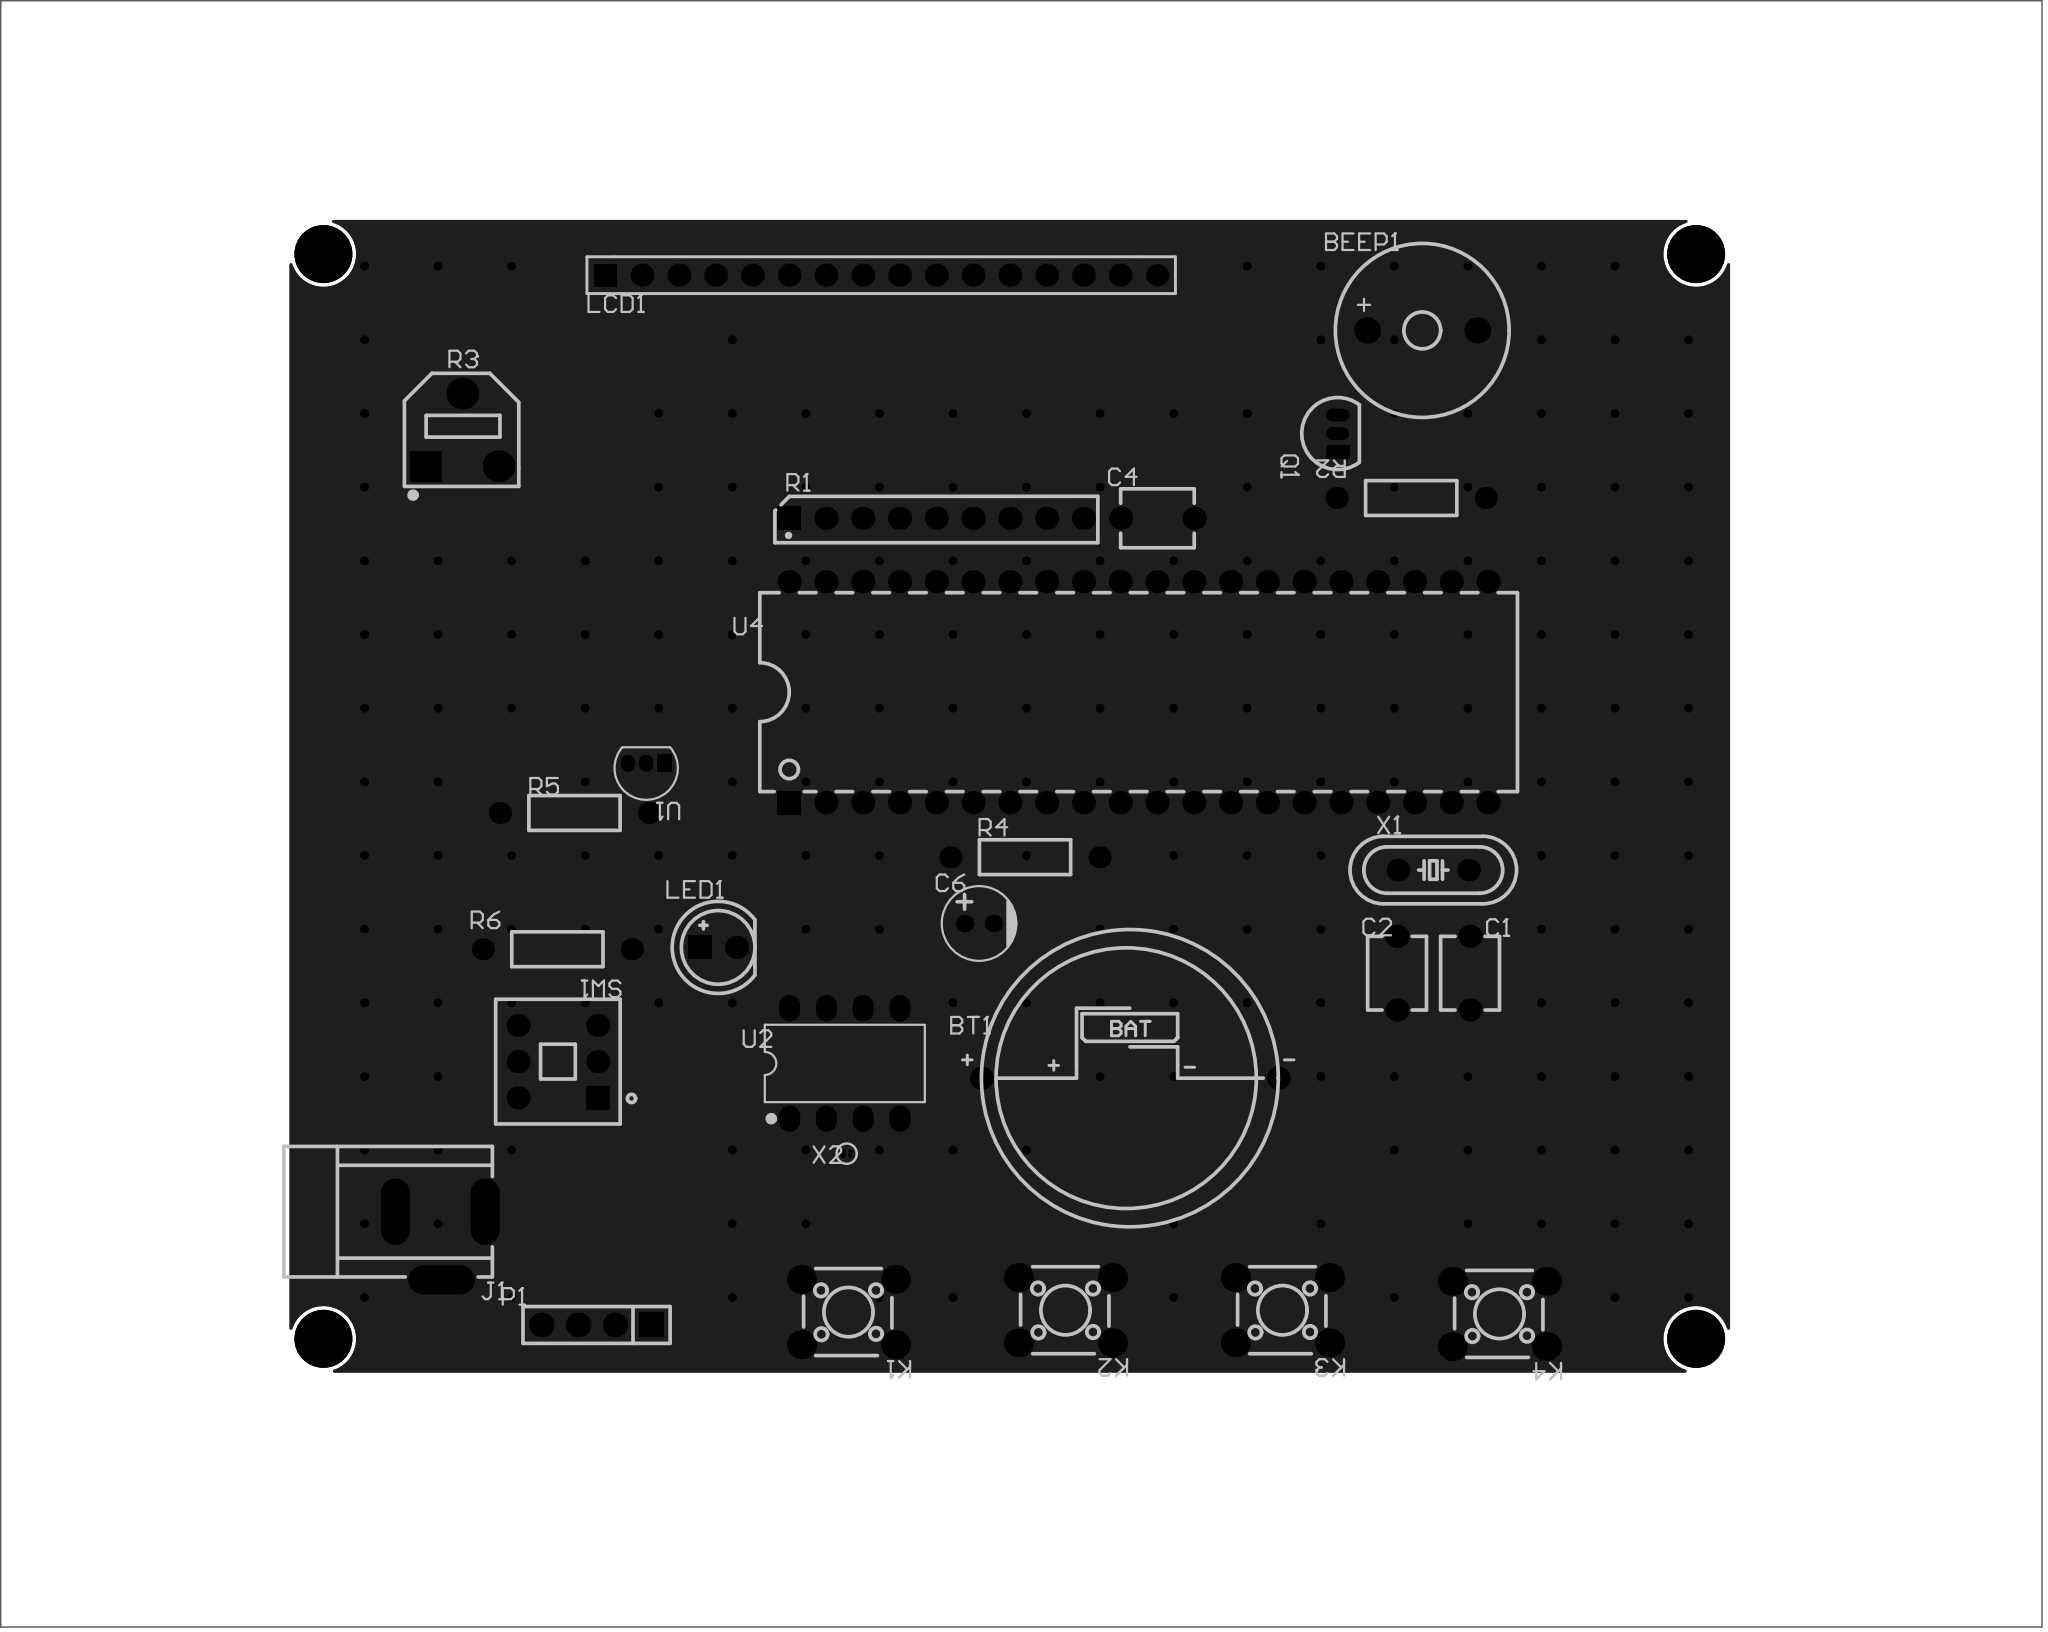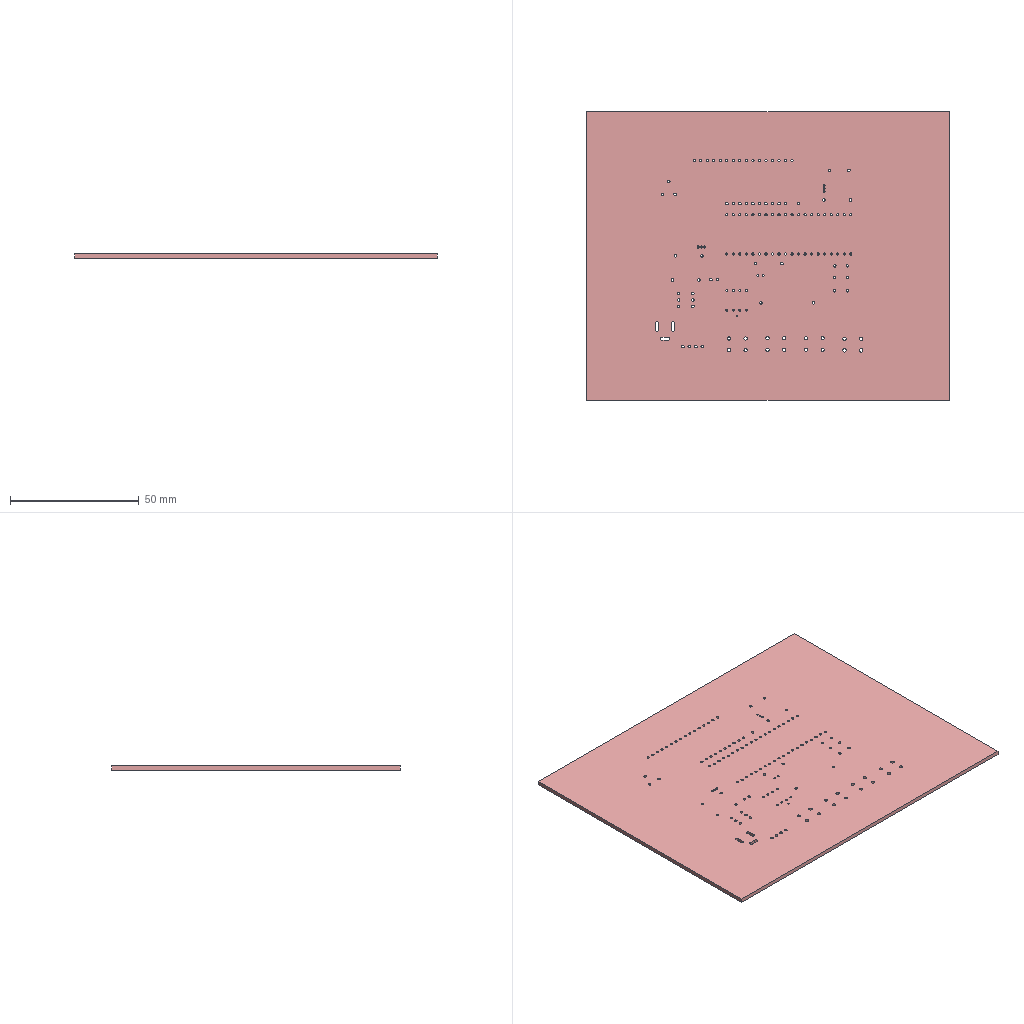Circuit board layout | Altium Designer | box 141 x 112.1 x 1.6 mm
Layer stack:
# Altium Designer layer stack of  (unit mm; dielectric type: 0 none, 1 core, 2 prepreg, 3 surface material)
index,name,kind,layer,copper_thickness_mm,dielectric_type,dielectric_thickness_mm,dielectric_material,dielectric_constant
0,Top Paste Mask Layer,other,,,,,,
1,Top Silkscreen Layer,other,,,,,,
2,Top Solder Mask Layer,dielectric,,,3,0.01,,3.3
3,Top Layer,copper,Top Layer,0.035,,,,
4,Dielectric1,dielectric,,,3,1.51,FR4,4.5
5,Bottom Layer,copper,Bottom Layer,0.035,,,,
6,Bottom Solder Mask Layer,dielectric,,,3,0.01,,3.3
7,Bottom Silkscreen Layer,other,,,,,,
8,Bottom Paste Mask Layer,other,,,,,,
# drill layer pairs: low layer,high layer
drill_pair,Top Layer,Bottom Layer
Part placement:
Designator,Comment,Layer,Footprint,Center-X(mm),Center-Y(mm),Rotation
BEEP1,,TopLayer,BUZ-TH_BD12.0-P7.60-D0.6-FD,168.021,159.258,0
BT1,Battery,TopLayer,BAT-TH_CR2032,147.828,107.696,0
C6,10uF,TopLayer,CAP-TH_BD5.0-P2.00-D0.6-FD,137.414,118.364,0
J1,,TopLayer,DC-005_2.5,100.203,96.139,180
LCD1,1602,TopLayer,HDR-M-2.54_1X16,130.655,163.068,0
Q1,8550,TopLayer,S8550P_TO-92,162.179,152.146,90
SW1,SWT,TopLayer,SW-TH_6P-L8.5-W8.5-P2.50-LS5.5-BL-2,108.331,108.839,90
U1,DS18B20,TopLayer,TO-92-3_L4.5-W3.5-P1.27-L,114.427,129.413,180
U2,DS1302,TopLayer,DIP-8_L10.9-W6.4-P2.54-LS7.6-BL,128.143,108.712,0
U4,STC89C52RC-40I-PDIP40,TopLayer,DIP-40_L52.0-W13.7-P2.54-LS15.2-BL,148.435,134.314,0
X2,32.768kHz,TopLayer,CRYSTAL-TH_BD1.4-P0.45-D0.2,128.27,102.489,180
X1,12M,TopLayer,HC-49S_L11.5-W4.7-P4.88,168.783,122.047,0
R1,,TopLayer,SIP-9_L22.3-W3.2-P2.54_KA2284-SIP-9,134.465,146.304,0
LED1,,TopLayer,LED-TH_5mm,119.396,116.713,0
P1,,TopLayer,HDR-TH_4P-P2.54-V-M,110.998,90.678,180
R2,1K,TopLayer,Res_1/4W,167.259,147.701,0
R4,10K,TopLayer,Res_1/4W,140.589,122.936,0
R5,4.7K,TopLayer,Res_1/4W,109.474,125.984,180
R6,1K,TopLayer,Res_1/4W,108.291,116.586,0
R3,103,TopLayer,RES-ADJ-SMD_RM065-V1,101.727,152.4,0
K1,,TopLayer,KEY-TH_4P-L6.0-W6.0-P4.50-LS6.50,128.397,91.567,180
K2,,TopLayer,KEY-TH_4P-L6.0-W6.0-P4.50-LS6.50,143.383,91.694,180
K3,,TopLayer,KEY-TH_4P-L6.0-W6.0-P4.50-LS6.50,158.369,91.694,180
K4,,TopLayer,KEY-TH_4P-L6.0-W6.0-P4.50-LS6.50,173.355,91.44,180
C4,0.1uF,TopLayer,CAP-TH_L5.0-W4.0-P5.00-D1.0,149.733,146.304,0
C1,30pF,TopLayer,CAP-TH_L5.0-W4.0-P5.00-D1.0,171.323,114.935,90
C2,30pF,TopLayer,CAP-TH_L5.0-W4.0-P5.00-D1.0,166.281,114.935,90
Pad and via stacks:
# Altium Designer via and pad stacks of  (unit mm). Each distinct definition once, with the count of objects using it.
# via: kind,start_layer,end_layer,hole_mm,diameter_mm,mode(0 simple;1 top-mid-bottom;2 full stack),diameter_per_layer,count,example_net
# pad: kind,layer,hole_mm,hole_type(0 round;1 square;2 slot),plating,top_size,top_shape(1 round;2 rect;3 octagon;9 rounded rect),mid_size,bottom_size,mode,footprint,size_per_layer,count,example
pad,Multi-Layer,1,0,plated,1.8x1.8,1,1.8x1.8,1.8x1.8,0,BUZ-TH_BD12.0-P7.60-D0.6-FD,,2,BEEP1.2
pad,Multi-Layer,1,0,plated,1.6x1.6,1,1.6x1.6,1.6x1.6,0,BAT-TH_CR2032,,2,BT1.1
pad,Multi-Layer,0.801,0,plated,1.202x1.202,1,1.202x1.202,1.202x1.202,0,CAP-TH_BD5.0-P2.00-D0.6-FD,,2,C6.1
pad,Multi-Layer,1.2,2,plated,2x4.6,1,2x4.6,2x4.6,0,DC-005_2.5,,2,J1.1
pad,Multi-Layer,1.2,2,plated,4.6x2,1,4.6x2,4.6x2,0,DC-005_2.5,,1,J1.3
pad,Multi-Layer,0.889,0,plated,1.575x1.575,1,1.575x1.575,1.575x1.575,0,HDR-M-2.54_1X16,,14,LCD1.15
pad,Multi-Layer,0.889,0,plated,1.575x1.575,2,1.575x1.575,1.575x1.575,0,HDR-M-2.54_1X16,,1,LCD1.1
pad,Multi-Layer,0.9144,0,plated,1.524x1.524,1,1.524x1.524,1.524x1.524,0,HDR-M-2.54_1X16,,1,LCD1.16
pad,Multi-Layer,0.7,0,plated,0.9x1.6,1,0.9x1.6,0.9x1.6,0,S8550P_TO-92,,2,Q1.3
pad,Multi-Layer,0.7,0,plated,0.9x1.6,2,0.9x1.6,0.9x1.6,0,S8550P_TO-92,,1,Q1.1
pad,Multi-Layer,1,0,plated,1.6x1.6,2,1.6x1.6,1.6x1.6,0,SW-TH_6P-L8.5-W8.5-P2.50-LS5.5-BL-2,,1,SW1.1
pad,Multi-Layer,1,0,plated,1.6x1.6,1,1.6x1.6,1.6x1.6,0,SW-TH_6P-L8.5-W8.5-P2.50-LS5.5-BL-2,,5,SW1.2
pad,Multi-Layer,0.7,2,plated,1x1.2,2,1x1.2,1x1.2,0,TO-92-3_L4.5-W3.5-P1.27-L,,1,U1.1
pad,Multi-Layer,0.7,2,plated,1x1.2,1,1x1.2,1x1.2,0,TO-92-3_L4.5-W3.5-P1.27-L,,2,U1.2
pad,Multi-Layer,0.8,0,plated,1.462x1.827,1,1.462x1.827,1.462x1.827,0,DIP-8_L10.9-W6.4-P2.54-LS7.6-BL,,8,U2.1
pad,Multi-Layer,0.889,0,plated,1.6x1.6,1,1.6x1.6,1.6x1.6,0,DIP-40_L52.0-W13.7-P2.54-LS15.2-BL,,39,U4.31
pad,Multi-Layer,0.889,0,plated,1.6x1.6,2,1.6x1.6,1.6x1.6,0,DIP-40_L52.0-W13.7-P2.54-LS15.2-BL,,1,U4.1
pad,Multi-Layer,0.27,0,plated,0.32x0.6,1,0.32x0.6,0.32x0.6,0,CRYSTAL-TH_BD1.4-P0.45-D0.2,,2,X2.1
pad,Multi-Layer,0.9,0,plated,1.56x1.56,1,1.56x1.56,1.56x1.56,0,HC-49S_L11.5-W4.7-P4.88,,2,X1.2
pad,Multi-Layer,1,0,plated,1.6x1.6,2,1.6x1.6,1.6x1.6,0,SIP-9_L22.3-W3.2-P2.54_KA2284-SIP-9,,1,R1.1
pad,Multi-Layer,1,0,plated,1.6x1.6,1,1.6x1.6,1.6x1.6,0,SIP-9_L22.3-W3.2-P2.54_KA2284-SIP-9,,8,R1.2
pad,Multi-Layer,1,0,plated,1.6x1.6,2,1.6x1.6,1.6x1.6,0,LED-TH_5mm,,1,LED1.1
pad,Multi-Layer,1,0,plated,1.6x1.6,1,1.6x1.6,1.6x1.6,0,LED-TH_5mm,,1,LED1.2
pad,Multi-Layer,1.1,0,plated,1.7x1.7,2,1.7x1.7,1.7x1.7,0,HDR-TH_4P-P2.54-V-M,,1,P1.1
pad,Multi-Layer,1.1,0,plated,1.7x1.7,1,1.7x1.7,1.7x1.7,0,HDR-TH_4P-P2.54-V-M,,3,P1.2
pad,Multi-Layer,1,0,plated,1.524x1.524,1,1.524x1.524,1.524x1.524,0,Res_1/4W,,8,R2.1
pad,Multi-Layer,1,0,plated,2.2x2.1,2,2.2x2.1,2.2x2.1,0,RES-ADJ-SMD_RM065-V1,,1,R3.1
pad,Multi-Layer,1,0,plated,2.2x2.2,1,2.2x2.2,2.2x2.2,0,RES-ADJ-SMD_RM065-V1,,2,R3.3
pad,Multi-Layer,1.3,0,plated,2x2,1,2x2,2x2,0,KEY-TH_4P-L6.0-W6.0-P4.50-LS6.50,,16,K1.4
pad,Multi-Layer,1,0,plated,1.6x1.6,1,1.6x1.6,1.6x1.6,0,CAP-TH_L5.0-W4.0-P5.00-D1.0,,6,C4.1
via,Top Layer,Bottom Layer,3,4,0,,4,
via,Top Layer,Bottom Layer,0.3048,0.61,0,,205,GND
Copper pours:
name,layer,net,type(0 solid;1 hatched;2 none)
Bottom Layer-GND,Bottom Layer,GND,0
Top Layer-GND,Top Layer,GND,0